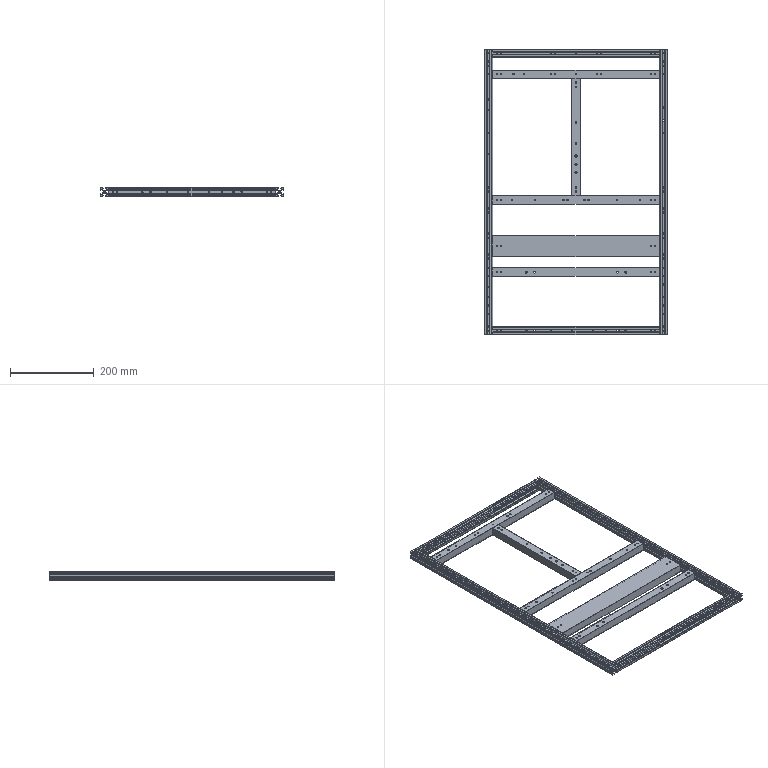Part | SolidWorks | features BaseBody 10 | 10 solids | 884 faces | box 438 x 682 x 20 mm | volume 641397 mm3 | cylinder 524 | plane 360 | commonest cylinder face diameters 3.2 x432 5 x48 3 x20 4.2 x12 5.2 x12